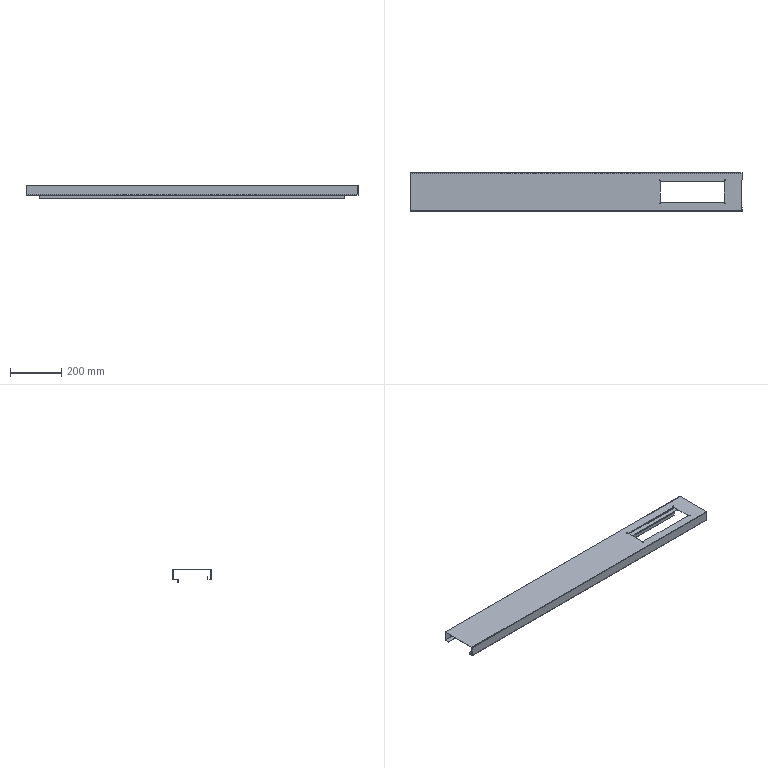Part | SolidWorks | features EdgeFlange 6, FlatPattern 1, ICE 1, SMBaseFlange 1, SheetMetal 1 | 1 solid | 70 faces | box 1298 x 150 x 53.8 mm | volume 411683 mm3 | plane 50 | cylinder 20 | commonest cylinder face diameters 3.9 x8 0.9 x6 3.3 x6